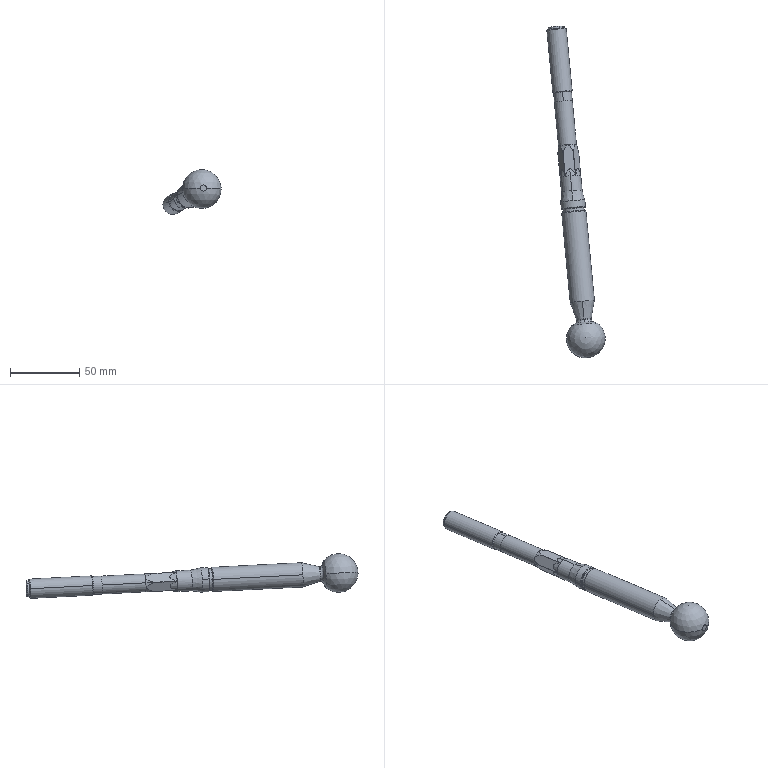Part | SolidWorks | features BaseBody 1 | 1 solid | 72 faces | box 42.008 x 239.227 x 32.291 mm | volume 49739 mm3 | cone 27 | plane 17 | cylinder 16 | torus 8 | sphere 4 | commonest cylinder face diameters 17.5 x4 11.5 x2 12.91 x2 12.94 x2 14 x2 14.95 x2